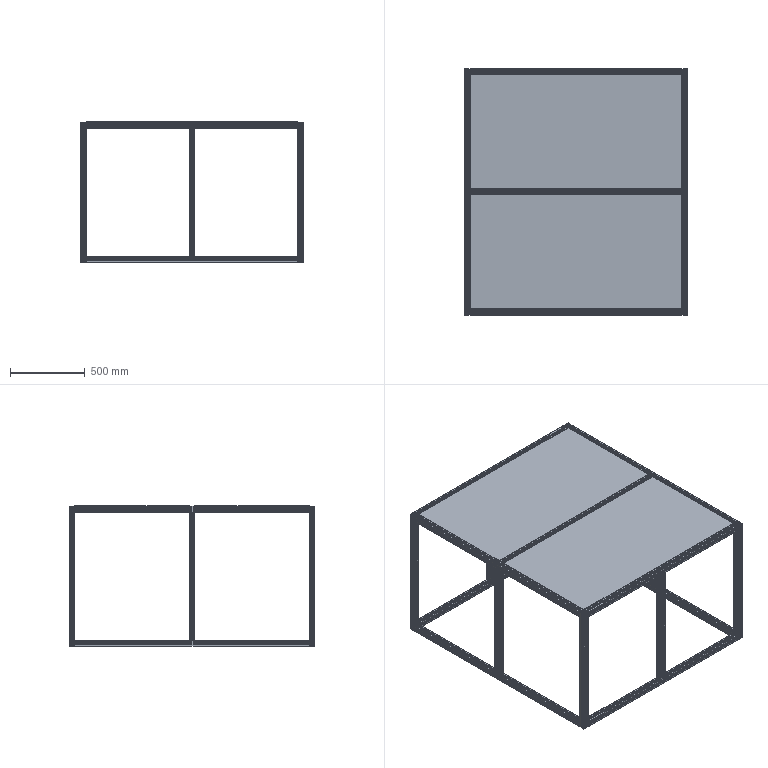Part | SolidWorks | features WeldCornerFeat 2, 3DProfileFeature 1, ICE 1, MirrorSolid 1, WeldMemberFeat 1, WeldmentFeature 1 | 19 solids | 1321 faces | box 1500 x 1650 x 942 mm | volume 12502911 mm3 | plane 1066 | cylinder 255 | commonest cylinder face diameters 2.2 x102 14 x85 1 x68